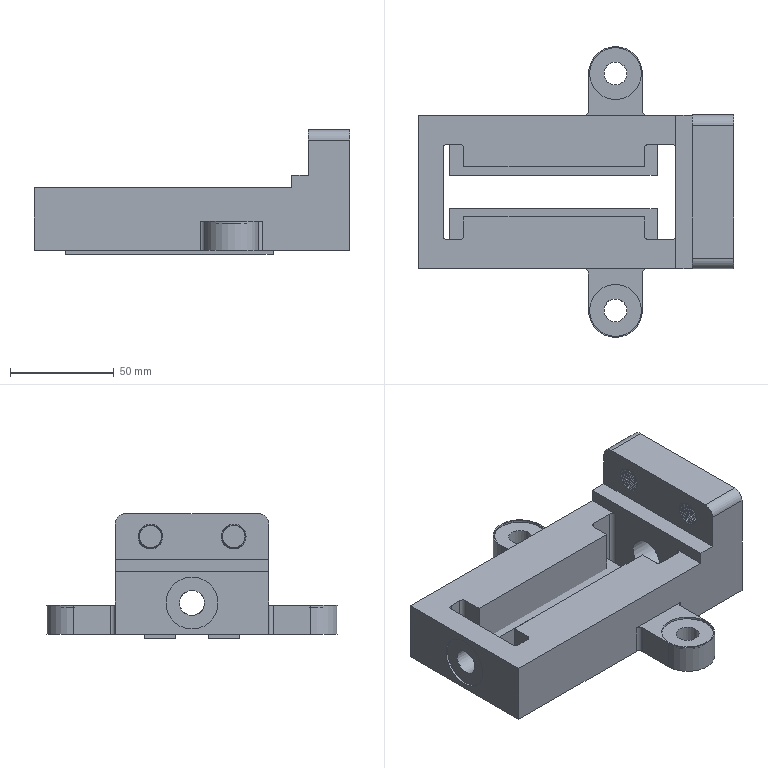Part | NX | features DATUM_CSYS 11, SKETCH 10, EXTRUDE 8, SIMPLE HOLE 4, HOLE PACKAGE 3, BLEND 2, THREADS 2 | 3 solids | 81 faces | box 152 x 140 x 60 mm | volume 327609 mm3 | plane 47 | cylinder 28 | spline 6 | commonest cylinder face diameters 4 x12 11 x4 12 x3 25 x3 10 x2 26 x2